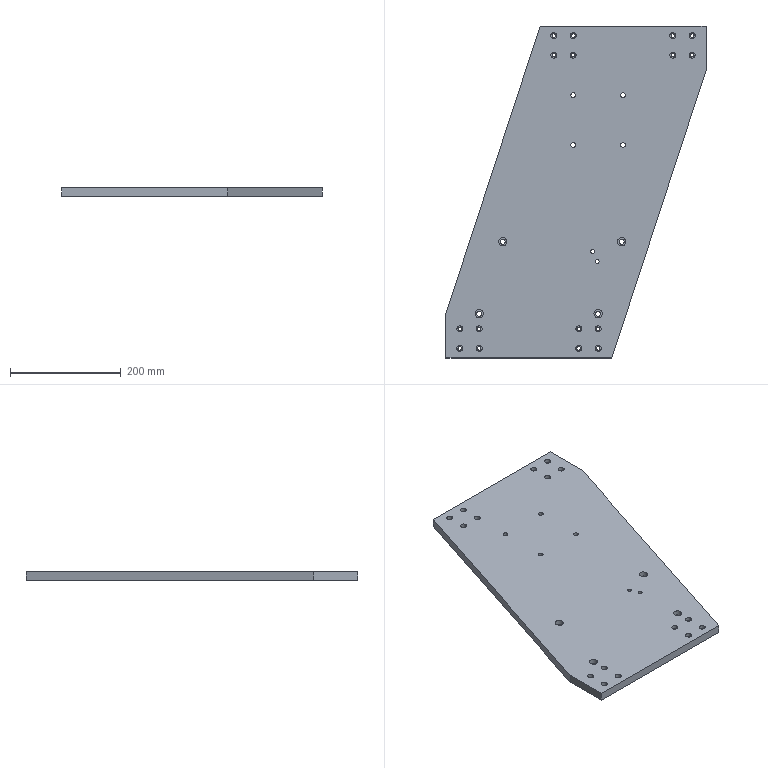Part | SolidWorks | features BaseBody 1 | 1 solid | 120 faces | box 470 x 600 x 15 mm | volume 2876789 mm3 | cylinder 92 | plane 28 | commonest cylinder face diameters 6.6 x32 11 x32 8.5 x8 9 x8 15 x8 6.8 x4